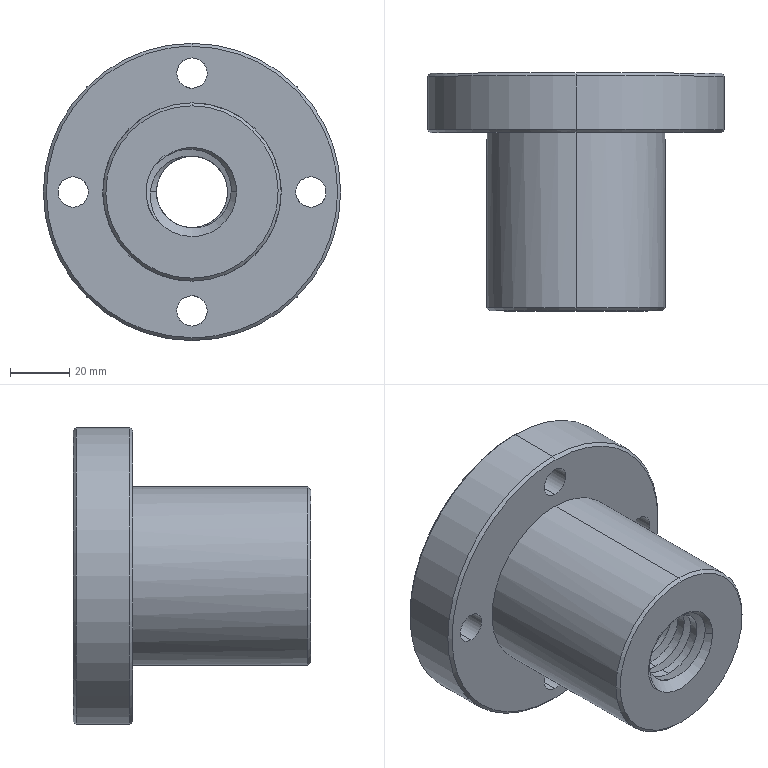Part | SolidWorks | features BaseBody 1 | 1 solid | 56 faces | box 100 x 80 x 100 mm | volume 274948 mm3 | cylinder 38 | cone 12 | plane 3 | spline 3 | commonest cylinder face diameters 24 x26 10.2 x8 60 x2 100 x2